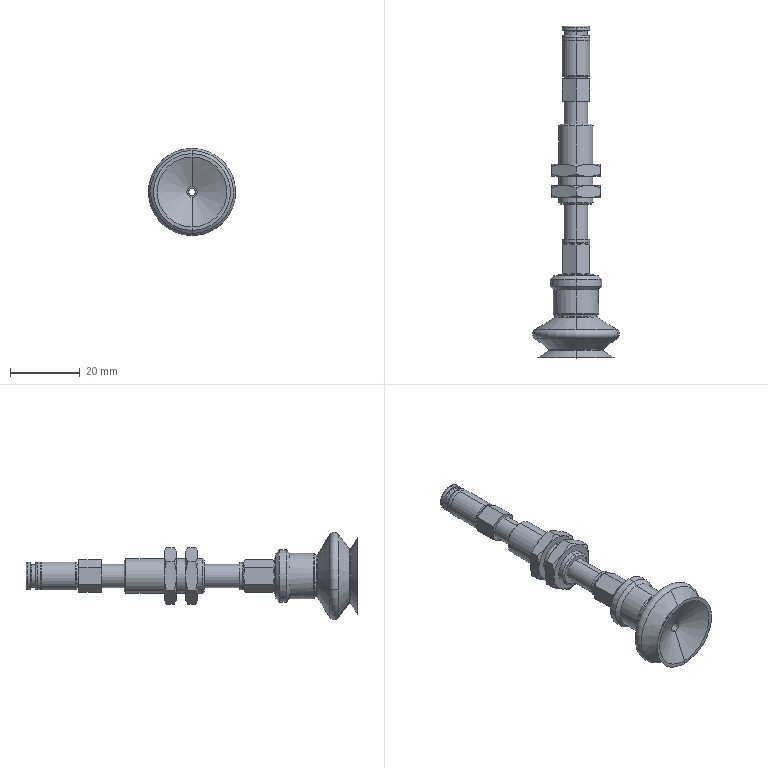Part | STEP file | KF-MISUMI_C-MPTBN-B20 suction cup | 5 solids | 211 faces | box 25 x 95.1 x 25 mm | volume 9058 mm3 | cone 76 | plane 65 | cylinder 40 | torus 30 | commonest cylinder face diameters 10 x8 6.7 x4 7.8 x4 8 x4 8.376 x4 2 x2